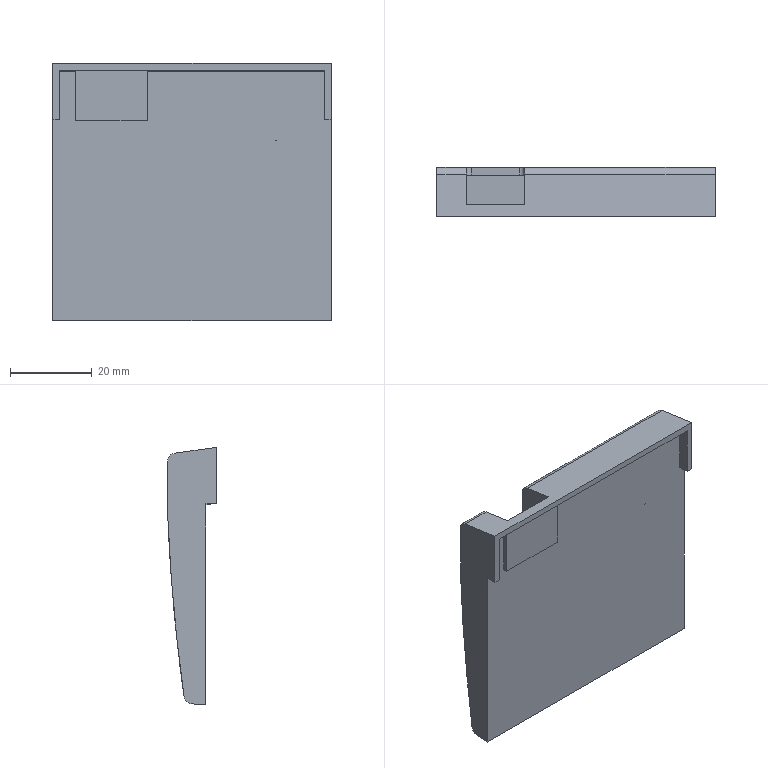Part | STEP file | ZXW735-L-95-04 | 2 solids | 176 faces | box 67.9 x 11.941 x 62.751 mm | volume 25948 mm3 | plane 111 | cylinder 36 | other 19 | sphere 4 | spline 4 | torus 2 | commonest cylinder face diameters 1 x20 4 x11 2.4 x2 3 x2 18.6 x1